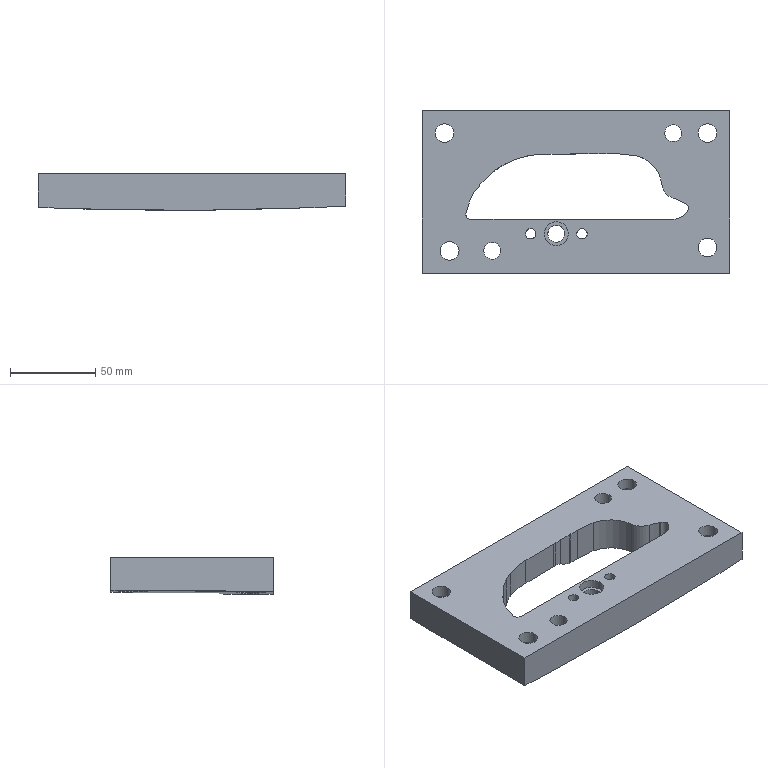Part | STEP file | 422_id1194_x_t | 1 solid | 75 faces | box 180 x 95 x 21.59 mm | volume 236336 mm3 | spline 36 | cylinder 21 | plane 18 | commonest cylinder face diameters 11 x6 17 x4 10 x3 4 x2 6 x2 6.1 x2